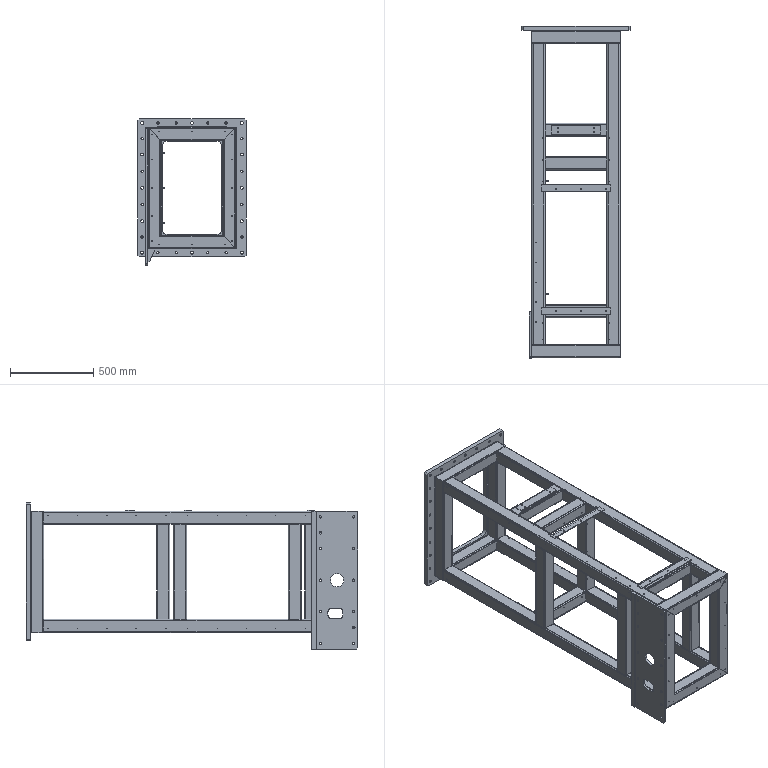Part | SolidWorks | features HoleWzd 25, WeldCornerFeat 15, ICE 11, Chamfer 8, WeldMemberFeat 3, Fillet 2, LPattern 2, MoveFace 2, 3DProfileFeature 1, WeldmentFeature 1 | 29 solids | 833 faces | box 650 x 1995 x 880 mm | volume 29715314 mm3 | cylinder 551 | plane 266 | cone 16 | commonest cylinder face diameters 3.3 x238 8 x92 16 x84 14 x54 6.8 x26 16.5 x24